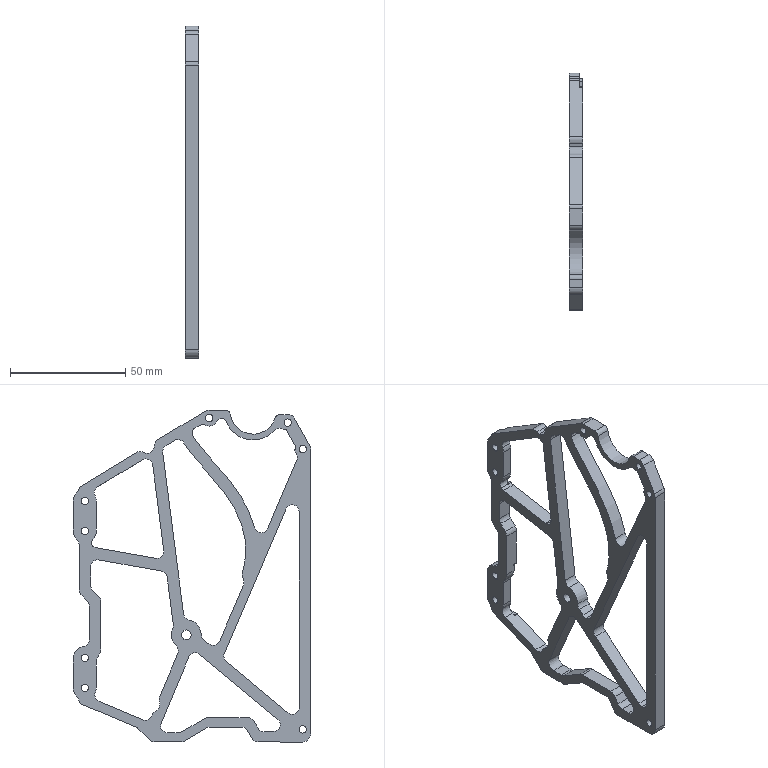Part | SolidWorks | features Fillet 3, ICE 2, Extrusion 1, HoleWzd 1 | 1 solid | 177 faces | box 6 x 103 x 144 mm | volume 23755 mm3 | cylinder 115 | plane 58 | cone 2 | spline 2 | commonest cylinder face diameters 6 x58 3.2 x16 2 x11 4 x8 10 x8 7 x5